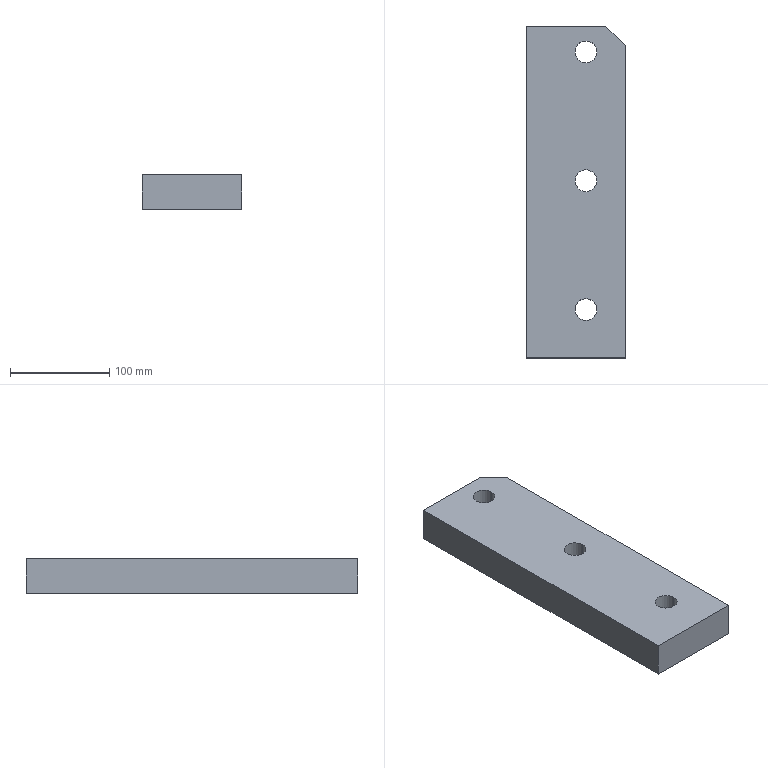Part | SolidWorks | features Chamfer 1, Extrusion 1, ICE 1 | 1 solid | 13 faces | box 100 x 335 x 35 mm | volume 1125586 mm3 | plane 7 | cylinder 6 | commonest cylinder face diameters 22 x6
STEP:
#1=CARTESIAN_POINT('',(-1.,141.328,0.));
#2=VERTEX_POINT('',#1);
#3=CARTESIAN_POINT('',(21.,141.328,0.));
#4=VERTEX_POINT('',#3);
#5=CARTESIAN_POINT('',(10.,141.328,0.));
#6=DIRECTION('',(0.,0.,1.));
#7=DIRECTION('',(1.,0.,0.));
#8=AXIS2_PLACEMENT_3D('',#5,#6,#7);
#9=CIRCLE('',#8,11.);
#10=EDGE_CURVE('',#2,#4,#9,.T.);
#11=ORIENTED_EDGE('',*,*,#10,.F.);
#12=CARTESIAN_POINT('',(-1.,141.328,35.));
#13=VERTEX_POINT('',#12);
#14=CARTESIAN_POINT('',(-1.,141.328,0.));
#15=DIRECTION('',(0.,0.,1.));
#16=VECTOR('',#15,1000.);
#17=LINE('',#14,#16);
#18=EDGE_CURVE('',#2,#13,#17,.T.);
#19=ORIENTED_EDGE('',*,*,#18,.T.);
#20=CARTESIAN_POINT('',(21.,141.328,35.));
#21=VERTEX_POINT('',#20);
#22=CARTESIAN_POINT('',(10.,141.328,35.));
#23=DIRECTION('',(0.,0.,-1.));
#24=DIRECTION('',(-1.,0.,0.));
#25=AXIS2_PLACEMENT_3D('',#22,#23,#24);
#26=CIRCLE('',#25,11.);
#27=EDGE_CURVE('',#21,#13,#26,.T.);
#28=ORIENTED_EDGE('',*,*,#27,.F.);
#29=CARTESIAN_POINT('',(21.,141.328,0.));
#30=DIRECTION('',(0.,0.,1.));
#31=VECTOR('',#30,1000.);
#32=LINE('',#29,#31);
#33=EDGE_CURVE('',#4,#21,#32,.T.);
#34=ORIENTED_EDGE('',*,*,#33,.F.);
#35=EDGE_LOOP('',(#11,#19,#28,#34));
#36=FACE_OUTER_BOUND('',#35,.T.);
#37=CARTESIAN_POINT('',(10.,141.328,0.));
#38=DIRECTION('',(0.,0.,1.));
#39=DIRECTION('',(1.,0.,0.));
#40=AXIS2_PLACEMENT_3D('',#37,#38,#39);
#41=CYLINDRICAL_SURFACE('',#40,11.);
#42=ADVANCED_FACE('',(#36),#41,.F.);
#43=CARTESIAN_POINT('',(-1.,-118.672,0.));
#44=VERTEX_POINT('',#43);
#45=CARTESIAN_POINT('',(21.,-118.672,0.));
#46=VERTEX_POINT('',#45);
#47=CARTESIAN_POINT('',(10.,-118.672,0.));
#48=DIRECTION('',(0.,0.,1.));
#49=DIRECTION('',(1.,0.,0.));
#50=AXIS2_PLACEMENT_3D('',#47,#48,#49);
#51=CIRCLE('',#50,11.);
#52=EDGE_CURVE('',#44,#46,#51,.T.);
#53=ORIENTED_EDGE('',*,*,#52,.F.);
#54=CARTESIAN_POINT('',(-1.,-118.672,35.));
#55=VERTEX_POINT('',#54);
#56=CARTESIAN_POINT('',(-1.,-118.672,0.));
#57=DIRECTION('',(0.,0.,1.));
#58=VECTOR('',#57,1000.);
#59=LINE('',#56,#58);
#60=EDGE_CURVE('',#44,#55,#59,.T.);
#61=ORIENTED_EDGE('',*,*,#60,.T.);
#62=CARTESIAN_POINT('',(21.,-118.672,35.));
#63=VERTEX_POINT('',#62);
#64=CARTESIAN_POINT('',(10.,-118.672,35.));
#65=DIRECTION('',(0.,0.,-1.));
#66=DIRECTION('',(-1.,0.,0.));
#67=AXIS2_PLACEMENT_3D('',#64,#65,#66);
#68=CIRCLE('',#67,11.);
#69=EDGE_CURVE('',#63,#55,#68,.T.);
#70=ORIENTED_EDGE('',*,*,#69,.F.);
#71=CARTESIAN_POINT('',(21.,-118.672,0.));
#72=DIRECTION('',(0.,0.,1.));
#73=VECTOR('',#72,1000.);
#74=LINE('',#71,#73);
#75=EDGE_CURVE('',#46,#63,#74,.T.);
#76=ORIENTED_EDGE('',*,*,#75,.F.);
#77=EDGE_LOOP('',(#53,#61,#70,#76));
#78=FACE_OUTER_BOUND('',#77,.T.);
#79=CARTESIAN_POINT('',(10.,-118.672,0.));
#80=DIRECTION('',(0.,0.,1.));
#81=DIRECTION('',(1.,0.,0.));
#82=AXIS2_PLACEMENT_3D('',#79,#80,#81);
#83=CYLINDRICAL_SURFACE('',#82,11.);
#84=ADVANCED_FACE('',(#78),#83,.F.);
#85=CARTESIAN_POINT('',(-1.,11.328,0.));
#86=VERTEX_POINT('',#85);
#87=CARTESIAN_POINT('',(21.,11.328,0.));
#88=VERTEX_POINT('',#87);
#89=CARTESIAN_POINT('',(10.,11.328,0.));
#90=DIRECTION('',(0.,0.,1.));
#91=DIRECTION('',(1.,0.,0.));
#92=AXIS2_PLACEMENT_3D('',#89,#90,#91);
#93=CIRCLE('',#92,11.);
#94=EDGE_CURVE('',#86,#88,#93,.T.);
#95=ORIENTED_EDGE('',*,*,#94,.F.);
#96=CARTESIAN_POINT('',(-1.,11.328,35.));
#97=VERTEX_POINT('',#96);
#98=CARTESIAN_POINT('',(-1.,11.328,0.));
#99=DIRECTION('',(0.,0.,1.));
#100=VECTOR('',#99,1000.);
#101=LINE('',#98,#100);
#102=EDGE_CURVE('',#86,#97,#101,.T.);
#103=ORIENTED_EDGE('',*,*,#102,.T.);
#104=CARTESIAN_POINT('',(21.,11.328,35.));
#105=VERTEX_POINT('',#104);
#106=CARTESIAN_POINT('',(10.,11.328,35.));
#107=DIRECTION('',(0.,0.,-1.));
#108=DIRECTION('',(-1.,0.,0.));
#109=AXIS2_PLACEMENT_3D('',#106,#107,#108);
#110=CIRCLE('',#109,11.);
#111=EDGE_CURVE('',#105,#97,#110,.T.);
#112=ORIENTED_EDGE('',*,*,#111,.F.);
#113=CARTESIAN_POINT('',(21.,11.328,0.));
#114=DIRECTION('',(0.,0.,1.));
#115=VECTOR('',#114,1000.);
#116=LINE('',#113,#115);
#117=EDGE_CURVE('',#88,#105,#116,.T.);
#118=ORIENTED_EDGE('',*,*,#117,.F.);
#119=EDGE_LOOP('',(#95,#103,#112,#118));
#120=FACE_OUTER_BOUND('',#119,.T.);
#121=CARTESIAN_POINT('',(10.,11.328,0.));
#122=DIRECTION('',(0.,0.,1.));
#123=DIRECTION('',(1.,0.,0.));
#124=AXIS2_PLACEMENT_3D('',#121,#122,#123);
#125=CYLINDRICAL_SURFACE('',#124,11.);
#126=ADVANCED_FACE('',(#120),#125,.F.);
#127=CARTESIAN_POINT('',(-50.,167.5,0.));
#128=VERTEX_POINT('',#127);
#129=CARTESIAN_POINT('',(-50.,-167.5,0.));
#130=VERTEX_POINT('',#129);
#131=CARTESIAN_POINT('',(-50.,167.5,0.));
#132=DIRECTION('',(0.,-1.,0.));
#133=VECTOR('',#132,1000.);
#134=LINE('',#131,#133);
#135=EDGE_CURVE('',#128,#130,#134,.T.);
#136=ORIENTED_EDGE('',*,*,#135,.T.);
#137=CARTESIAN_POINT('',(-50.,-167.5,35.));
#138=VERTEX_POINT('',#137);
#139=CARTESIAN_POINT('',(-50.,-167.5,35.));
#140=DIRECTION('',(0.,0.,-1.));
#141=VECTOR('',#140,1000.);
#142=LINE('',#139,#141);
#143=EDGE_CURVE('',#138,#130,#142,.T.);
#144=ORIENTED_EDGE('',*,*,#143,.F.);
#145=CARTESIAN_POINT('',(-50.,167.5,35.));
#146=VERTEX_POINT('',#145);
#147=CARTESIAN_POINT('',(-50.,167.5,35.));
#148=DIRECTION('',(0.,-1.,0.));
#149=VECTOR('',#148,1000.);
#150=LINE('',#147,#149);
#151=EDGE_CURVE('',#146,#138,#150,.T.);
#152=ORIENTED_EDGE('',*,*,#151,.F.);
#153=CARTESIAN_POINT('',(-50.,167.5,35.));
#154=DIRECTION('',(0.,0.,-1.));
#155=VECTOR('',#154,1000.);
#156=LINE('',#153,#155);
#157=EDGE_CURVE('',#146,#128,#156,.T.);
#158=ORIENTED_EDGE('',*,*,#157,.T.);
#159=EDGE_LOOP('',(#136,#144,#152,#158));
#160=FACE_OUTER_BOUND('',#159,.T.);
#161=CARTESIAN_POINT('',(-50.,167.5,35.));
#162=DIRECTION('',(1.,0.,0.));
#163=DIRECTION('',(0.,1.,0.));
#164=AXIS2_PLACEMENT_3D('',#161,#162,#163);
#165=PLANE('',#164);
#166=ADVANCED_FACE('',(#160),#165,.F.);
#167=CARTESIAN_POINT('',(50.,-167.5,0.));
#168=VERTEX_POINT('',#167);
#169=CARTESIAN_POINT('',(50.,-167.5,0.));
#170=DIRECTION('',(1.,0.,0.));
#171=VECTOR('',#170,1000.);
#172=LINE('',#169,#171);
#173=EDGE_CURVE('',#130,#168,#172,.T.);
#174=ORIENTED_EDGE('',*,*,#173,.T.);
#175=CARTESIAN_POINT('',(50.,-167.5,35.));
#176=VERTEX_POINT('',#175);
#177=CARTESIAN_POINT('',(50.,-167.5,35.));
#178=DIRECTION('',(0.,0.,-1.));
#179=VECTOR('',#178,1000.);
#180=LINE('',#177,#179);
#181=EDGE_CURVE('',#176,#168,#180,.T.);
#182=ORIENTED_EDGE('',*,*,#181,.F.);
#183=CARTESIAN_POINT('',(50.,-167.5,35.));
#184=DIRECTION('',(1.,0.,0.));
#185=VECTOR('',#184,1000.);
#186=LINE('',#183,#185);
#187=EDGE_CURVE('',#138,#176,#186,.T.);
#188=ORIENTED_EDGE('',*,*,#187,.F.);
#189=ORIENTED_EDGE('',*,*,#143,.T.);
#190=EDGE_LOOP('',(#174,#182,#188,#189));
#191=FACE_OUTER_BOUND('',#190,.T.);
#192=CARTESIAN_POINT('',(50.,-167.5,35.));
#193=DIRECTION('',(0.,1.,0.));
#194=DIRECTION('',(0.,0.,1.));
#195=AXIS2_PLACEMENT_3D('',#192,#193,#194);
#196=PLANE('',#195);
#197=ADVANCED_FACE('',(#191),#196,.F.);
#198=CARTESIAN_POINT('',(50.,147.5,0.));
#199=VERTEX_POINT('',#198);
#200=CARTESIAN_POINT('',(50.,167.5,0.));
#201=DIRECTION('',(0.,1.,0.));
#202=VECTOR('',#201,1000.);
#203=LINE('',#200,#202);
#204=EDGE_CURVE('',#168,#199,#203,.T.);
#205=ORIENTED_EDGE('',*,*,#204,.T.);
#206=CARTESIAN_POINT('',(50.,147.5,35.));
#207=VERTEX_POINT('',#206);
#208=CARTESIAN_POINT('',(50.,147.5,35.));
#209=DIRECTION('',(0.,0.,1.));
#210=VECTOR('',#209,1000.);
#211=LINE('',#208,#210);
#212=EDGE_CURVE('',#199,#207,#211,.T.);
#213=ORIENTED_EDGE('',*,*,#212,.T.);
#214=CARTESIAN_POINT('',(50.,167.5,35.));
#215=DIRECTION('',(0.,1.,0.));
#216=VECTOR('',#215,1000.);
#217=LINE('',#214,#216);
#218=EDGE_CURVE('',#176,#207,#217,.T.);
#219=ORIENTED_EDGE('',*,*,#218,.F.);
#220=ORIENTED_EDGE('',*,*,#181,.T.);
#221=EDGE_LOOP('',(#205,#213,#219,#220));
#222=FACE_OUTER_BOUND('',#221,.T.);
#223=CARTESIAN_POINT('',(50.,167.5,35.));
#224=DIRECTION('',(-1.,0.,0.));
#225=DIRECTION('',(0.,-1.,0.));
#226=AXIS2_PLACEMENT_3D('',#223,#224,#225);
#227=PLANE('',#226);
#228=ADVANCED_FACE('',(#222),#227,.F.);
#229=CARTESIAN_POINT('',(30.,167.5,35.));
#230=VERTEX_POINT('',#229);
#231=CARTESIAN_POINT('',(50.,167.5,35.));
#232=DIRECTION('',(-1.,0.,0.));
#233=VECTOR('',#232,1000.);
#234=LINE('',#231,#233);
#235=EDGE_CURVE('',#230,#146,#234,.T.);
#236=ORIENTED_EDGE('',*,*,#235,.F.);
#237=CARTESIAN_POINT('',(30.,167.5,0.));
#238=VERTEX_POINT('',#237);
#239=CARTESIAN_POINT('',(30.,167.5,35.));
#240=DIRECTION('',(0.,0.,-1.));
#241=VECTOR('',#240,1000.);
#242=LINE('',#239,#241);
#243=EDGE_CURVE('',#230,#238,#242,.T.);
#244=ORIENTED_EDGE('',*,*,#243,.T.);
#245=CARTESIAN_POINT('',(50.,167.5,0.));
#246=DIRECTION('',(-1.,0.,0.));
#247=VECTOR('',#246,1000.);
#248=LINE('',#245,#247);
#249=EDGE_CURVE('',#238,#128,#248,.T.);
#250=ORIENTED_EDGE('',*,*,#249,.T.);
#251=ORIENTED_EDGE('',*,*,#157,.F.);
#252=EDGE_LOOP('',(#236,#244,#250,#251));
#253=FACE_OUTER_BOUND('',#252,.T.);
#254=CARTESIAN_POINT('',(50.,167.5,35.));
#255=DIRECTION('',(0.,-1.,0.));
#256=DIRECTION('',(0.,0.,-1.));
#257=AXIS2_PLACEMENT_3D('',#254,#255,#256);
#258=PLANE('',#257);
#259=ADVANCED_FACE('',(#253),#258,.F.);
#260=ORIENTED_EDGE('',*,*,#27,.T.);
#261=CARTESIAN_POINT('',(10.,141.328,35.));
#262=DIRECTION('',(0.,0.,-1.));
#263=DIRECTION('',(-1.,0.,0.));
#264=AXIS2_PLACEMENT_3D('',#261,#262,#263);
#265=CIRCLE('',#264,11.);
#266=EDGE_CURVE('',#13,#21,#265,.T.);
#267=ORIENTED_EDGE('',*,*,#266,.T.);
#268=EDGE_LOOP('',(#260,#267));
#269=FACE_BOUND('',#268,.T.);
#270=ORIENTED_EDGE('',*,*,#69,.T.);
#271=CARTESIAN_POINT('',(10.,-118.672,35.));
#272=DIRECTION('',(0.,0.,-1.));
#273=DIRECTION('',(-1.,0.,0.));
#274=AXIS2_PLACEMENT_3D('',#271,#272,#273);
#275=CIRCLE('',#274,11.);
#276=EDGE_CURVE('',#55,#63,#275,.T.);
#277=ORIENTED_EDGE('',*,*,#276,.T.);
#278=EDGE_LOOP('',(#270,#277));
#279=FACE_BOUND('',#278,.T.);
#280=ORIENTED_EDGE('',*,*,#111,.T.);
#281=CARTESIAN_POINT('',(10.,11.328,35.));
#282=DIRECTION('',(0.,0.,-1.));
#283=DIRECTION('',(-1.,0.,0.));
#284=AXIS2_PLACEMENT_3D('',#281,#282,#283);
#285=CIRCLE('',#284,11.);
#286=EDGE_CURVE('',#97,#105,#285,.T.);
#287=ORIENTED_EDGE('',*,*,#286,.T.);
#288=EDGE_LOOP('',(#280,#287));
#289=FACE_BOUND('',#288,.T.);
#290=ORIENTED_EDGE('',*,*,#218,.T.);
#291=CARTESIAN_POINT('',(30.,167.5,35.));
#292=DIRECTION('',(-0.7071,0.7071,0.));
#293=VECTOR('',#292,1000.);
#294=LINE('',#291,#293);
#295=EDGE_CURVE('',#207,#230,#294,.T.);
#296=ORIENTED_EDGE('',*,*,#295,.T.);
#297=ORIENTED_EDGE('',*,*,#235,.T.);
#298=ORIENTED_EDGE('',*,*,#151,.T.);
#299=ORIENTED_EDGE('',*,*,#187,.T.);
#300=EDGE_LOOP('',(#290,#296,#297,#298,#299));
#301=FACE_OUTER_BOUND('',#300,.T.);
#302=CARTESIAN_POINT('',(0.,0.,35.));
#303=DIRECTION('',(0.,0.,-1.));
#304=DIRECTION('',(-1.,0.,0.));
#305=AXIS2_PLACEMENT_3D('',#302,#303,#304);
#306=PLANE('',#305);
#307=ADVANCED_FACE('',(#269,#279,#289,#301),#306,.F.);
#308=CARTESIAN_POINT('',(10.,141.328,0.));
#309=DIRECTION('',(0.,0.,1.));
#310=DIRECTION('',(1.,0.,0.));
#311=AXIS2_PLACEMENT_3D('',#308,#309,#310);
#312=CIRCLE('',#311,11.);
#313=EDGE_CURVE('',#4,#2,#312,.T.);
#314=ORIENTED_EDGE('',*,*,#313,.T.);
#315=ORIENTED_EDGE('',*,*,#10,.T.);
#316=EDGE_LOOP('',(#314,#315));
#317=FACE_BOUND('',#316,.T.);
#318=CARTESIAN_POINT('',(10.,-118.672,0.));
#319=DIRECTION('',(0.,0.,1.));
#320=DIRECTION('',(1.,0.,0.));
#321=AXIS2_PLACEMENT_3D('',#318,#319,#320);
#322=CIRCLE('',#321,11.);
#323=EDGE_CURVE('',#46,#44,#322,.T.);
#324=ORIENTED_EDGE('',*,*,#323,.T.);
#325=ORIENTED_EDGE('',*,*,#52,.T.);
#326=EDGE_LOOP('',(#324,#325));
#327=FACE_BOUND('',#326,.T.);
#328=CARTESIAN_POINT('',(10.,11.328,0.));
#329=DIRECTION('',(0.,0.,1.));
#330=DIRECTION('',(1.,0.,0.));
#331=AXIS2_PLACEMENT_3D('',#328,#329,#330);
#332=CIRCLE('',#331,11.);
#333=EDGE_CURVE('',#88,#86,#332,.T.);
#334=ORIENTED_EDGE('',*,*,#333,.T.);
#335=ORIENTED_EDGE('',*,*,#94,.T.);
#336=EDGE_LOOP('',(#334,#335));
#337=FACE_BOUND('',#336,.T.);
#338=ORIENTED_EDGE('',*,*,#249,.F.);
#339=CARTESIAN_POINT('',(98.75,98.75,0.));
#340=DIRECTION('',(0.7071,-0.7071,0.));
#341=VECTOR('',#340,1000.);
#342=LINE('',#339,#341);
#343=EDGE_CURVE('',#238,#199,#342,.T.);
#344=ORIENTED_EDGE('',*,*,#343,.T.);
#345=ORIENTED_EDGE('',*,*,#204,.F.);
#346=ORIENTED_EDGE('',*,*,#173,.F.);
#347=ORIENTED_EDGE('',*,*,#135,.F.);
#348=EDGE_LOOP('',(#338,#344,#345,#346,#347));
#349=FACE_OUTER_BOUND('',#348,.T.);
#350=CARTESIAN_POINT('',(0.,0.,0.));
#351=DIRECTION('',(0.,0.,-1.));
#352=DIRECTION('',(-1.,0.,0.));
#353=AXIS2_PLACEMENT_3D('',#350,#351,#352);
#354=PLANE('',#353);
#355=ADVANCED_FACE('',(#317,#327,#337,#349),#354,.T.);
#356=ORIENTED_EDGE('',*,*,#295,.F.);
#357=ORIENTED_EDGE('',*,*,#212,.F.);
#358=ORIENTED_EDGE('',*,*,#343,.F.);
#359=ORIENTED_EDGE('',*,*,#243,.F.);
#360=EDGE_LOOP('',(#356,#357,#358,#359));
#361=FACE_OUTER_BOUND('',#360,.T.);
#362=CARTESIAN_POINT('',(30.,167.5,35.));
#363=DIRECTION('',(-0.7071,-0.7071,0.));
#364=DIRECTION('',(0.,0.,-1.));
#365=AXIS2_PLACEMENT_3D('',#362,#363,#364);
#366=PLANE('',#365);
#367=ADVANCED_FACE('',(#361),#366,.F.);
#368=ORIENTED_EDGE('',*,*,#102,.F.);
#369=ORIENTED_EDGE('',*,*,#333,.F.);
#370=ORIENTED_EDGE('',*,*,#117,.T.);
#371=ORIENTED_EDGE('',*,*,#286,.F.);
#372=EDGE_LOOP('',(#368,#369,#370,#371));
#373=FACE_OUTER_BOUND('',#372,.T.);
#374=CARTESIAN_POINT('',(10.,11.328,0.));
#375=DIRECTION('',(0.,0.,1.));
#376=DIRECTION('',(1.,0.,0.));
#377=AXIS2_PLACEMENT_3D('',#374,#375,#376);
#378=CYLINDRICAL_SURFACE('',#377,11.);
#379=ADVANCED_FACE('',(#373),#378,.F.);
#380=ORIENTED_EDGE('',*,*,#60,.F.);
#381=ORIENTED_EDGE('',*,*,#323,.F.);
#382=ORIENTED_EDGE('',*,*,#75,.T.);
#383=ORIENTED_EDGE('',*,*,#276,.F.);
#384=EDGE_LOOP('',(#380,#381,#382,#383));
#385=FACE_OUTER_BOUND('',#384,.T.);
#386=CARTESIAN_POINT('',(10.,-118.672,0.));
#387=DIRECTION('',(0.,0.,1.));
#388=DIRECTION('',(1.,0.,0.));
#389=AXIS2_PLACEMENT_3D('',#386,#387,#388);
#390=CYLINDRICAL_SURFACE('',#389,11.);
#391=ADVANCED_FACE('',(#385),#390,.F.);
#392=ORIENTED_EDGE('',*,*,#18,.F.);
#393=ORIENTED_EDGE('',*,*,#313,.F.);
#394=ORIENTED_EDGE('',*,*,#33,.T.);
#395=ORIENTED_EDGE('',*,*,#266,.F.);
#396=EDGE_LOOP('',(#392,#393,#394,#395));
#397=FACE_OUTER_BOUND('',#396,.T.);
#398=CARTESIAN_POINT('',(10.,141.328,0.));
#399=DIRECTION('',(0.,0.,1.));
#400=DIRECTION('',(1.,0.,0.));
#401=AXIS2_PLACEMENT_3D('',#398,#399,#400);
#402=CYLINDRICAL_SURFACE('',#401,11.);
#403=ADVANCED_FACE('',(#397),#402,.F.);
#404=CLOSED_SHELL('',(#42,#84,#126,#166,#197,#228,#259,#307,#355,#367,#379,#391,#403));
#405=MANIFOLD_SOLID_BREP('',#404);
#406=CARTESIAN_POINT('',(0.,0.,0.));
#407=DIRECTION('',(0.,0.,1.));
#408=DIRECTION('',(1.,0.,0.));
#409=AXIS2_PLACEMENT_3D('',#406,#407,#408);
#410=(LENGTH_UNIT()NAMED_UNIT(*)SI_UNIT(.MILLI.,.METRE.));
#411=UNCERTAINTY_MEASURE_WITH_UNIT(LENGTH_MEASURE(0.00001),#410,'','');
#412=(NAMED_UNIT(*)PLANE_ANGLE_UNIT()SI_UNIT($,.RADIAN.));
#413=(NAMED_UNIT(*)SI_UNIT($,.STERADIAN.)SOLID_ANGLE_UNIT());
#414=(GEOMETRIC_REPRESENTATION_CONTEXT(3)GLOBAL_UNCERTAINTY_ASSIGNED_CONTEXT((#411))GLOBAL_UNIT_ASSIGNED_CONTEXT((#410,#412,#413))REPRESENTATION_CONTEXT('',''));
#415=ADVANCED_BREP_SHAPE_REPRESENTATION('',(#405,#409),#414);